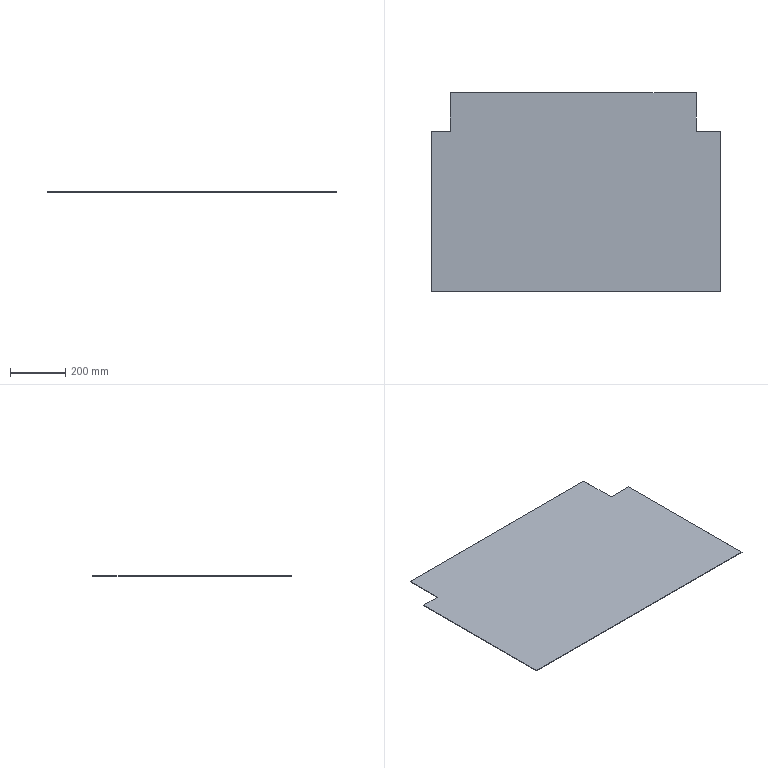Part | SolidWorks | 1 solid | 10 faces | box 1050 x 720 x 2 mm | volume 1467200 mm3 | plane 10
STEP:
#1=CARTESIAN_POINT('',(445.,655.,0.));
#2=VERTEX_POINT('',#1);
#3=CARTESIAN_POINT('',(445.,795.,0.));
#4=VERTEX_POINT('',#3);
#5=CARTESIAN_POINT('',(445.,795.,0.));
#6=DIRECTION('',(0.,1.,0.));
#7=VECTOR('',#6,1000.);
#8=LINE('',#5,#7);
#9=EDGE_CURVE('',#2,#4,#8,.T.);
#10=ORIENTED_EDGE('',*,*,#9,.T.);
#11=CARTESIAN_POINT('',(445.,795.,2.));
#12=VERTEX_POINT('',#11);
#13=CARTESIAN_POINT('',(445.,795.,2.));
#14=DIRECTION('',(0.,0.,-1.));
#15=VECTOR('',#14,1000.);
#16=LINE('',#13,#15);
#17=EDGE_CURVE('',#12,#4,#16,.T.);
#18=ORIENTED_EDGE('',*,*,#17,.F.);
#19=CARTESIAN_POINT('',(445.,655.,2.));
#20=VERTEX_POINT('',#19);
#21=CARTESIAN_POINT('',(445.,795.,2.));
#22=DIRECTION('',(0.,1.,0.));
#23=VECTOR('',#22,1000.);
#24=LINE('',#21,#23);
#25=EDGE_CURVE('',#20,#12,#24,.T.);
#26=ORIENTED_EDGE('',*,*,#25,.F.);
#27=CARTESIAN_POINT('',(445.,655.,2.));
#28=DIRECTION('',(0.,0.,-1.));
#29=VECTOR('',#28,1000.);
#30=LINE('',#27,#29);
#31=EDGE_CURVE('',#20,#2,#30,.T.);
#32=ORIENTED_EDGE('',*,*,#31,.T.);
#33=EDGE_LOOP('',(#10,#18,#26,#32));
#34=FACE_OUTER_BOUND('',#33,.T.);
#35=CARTESIAN_POINT('',(445.,795.,2.));
#36=DIRECTION('',(-1.,0.,0.));
#37=DIRECTION('',(0.,0.,1.));
#38=AXIS2_PLACEMENT_3D('',#35,#36,#37);
#39=PLANE('',#38);
#40=ADVANCED_FACE('',(#34),#39,.F.);
#41=CARTESIAN_POINT('',(-445.,795.,0.));
#42=VERTEX_POINT('',#41);
#43=CARTESIAN_POINT('',(-445.,795.,0.));
#44=DIRECTION('',(-1.,0.,0.));
#45=VECTOR('',#44,1000.);
#46=LINE('',#43,#45);
#47=EDGE_CURVE('',#4,#42,#46,.T.);
#48=ORIENTED_EDGE('',*,*,#47,.T.);
#49=CARTESIAN_POINT('',(-445.,795.,2.));
#50=VERTEX_POINT('',#49);
#51=CARTESIAN_POINT('',(-445.,795.,2.));
#52=DIRECTION('',(0.,0.,-1.));
#53=VECTOR('',#52,1000.);
#54=LINE('',#51,#53);
#55=EDGE_CURVE('',#50,#42,#54,.T.);
#56=ORIENTED_EDGE('',*,*,#55,.F.);
#57=CARTESIAN_POINT('',(-445.,795.,2.));
#58=DIRECTION('',(-1.,0.,0.));
#59=VECTOR('',#58,1000.);
#60=LINE('',#57,#59);
#61=EDGE_CURVE('',#12,#50,#60,.T.);
#62=ORIENTED_EDGE('',*,*,#61,.F.);
#63=ORIENTED_EDGE('',*,*,#17,.T.);
#64=EDGE_LOOP('',(#48,#56,#62,#63));
#65=FACE_OUTER_BOUND('',#64,.T.);
#66=CARTESIAN_POINT('',(-445.,795.,2.));
#67=DIRECTION('',(0.,-1.,0.));
#68=DIRECTION('',(0.,0.,-1.));
#69=AXIS2_PLACEMENT_3D('',#66,#67,#68);
#70=PLANE('',#69);
#71=ADVANCED_FACE('',(#65),#70,.F.);
#72=CARTESIAN_POINT('',(-445.,655.,0.));
#73=VERTEX_POINT('',#72);
#74=CARTESIAN_POINT('',(-445.,795.,0.));
#75=DIRECTION('',(0.,-1.,0.));
#76=VECTOR('',#75,1000.);
#77=LINE('',#74,#76);
#78=EDGE_CURVE('',#42,#73,#77,.T.);
#79=ORIENTED_EDGE('',*,*,#78,.T.);
#80=CARTESIAN_POINT('',(-445.,655.,2.));
#81=VERTEX_POINT('',#80);
#82=CARTESIAN_POINT('',(-445.,655.,2.));
#83=DIRECTION('',(0.,0.,-1.));
#84=VECTOR('',#83,1000.);
#85=LINE('',#82,#84);
#86=EDGE_CURVE('',#81,#73,#85,.T.);
#87=ORIENTED_EDGE('',*,*,#86,.F.);
#88=CARTESIAN_POINT('',(-445.,795.,2.));
#89=DIRECTION('',(0.,-1.,0.));
#90=VECTOR('',#89,1000.);
#91=LINE('',#88,#90);
#92=EDGE_CURVE('',#50,#81,#91,.T.);
#93=ORIENTED_EDGE('',*,*,#92,.F.);
#94=ORIENTED_EDGE('',*,*,#55,.T.);
#95=EDGE_LOOP('',(#79,#87,#93,#94));
#96=FACE_OUTER_BOUND('',#95,.T.);
#97=CARTESIAN_POINT('',(-445.,795.,2.));
#98=DIRECTION('',(1.,0.,0.));
#99=DIRECTION('',(0.,0.,-1.));
#100=AXIS2_PLACEMENT_3D('',#97,#98,#99);
#101=PLANE('',#100);
#102=ADVANCED_FACE('',(#96),#101,.F.);
#103=CARTESIAN_POINT('',(-515.,655.,0.));
#104=VERTEX_POINT('',#103);
#105=CARTESIAN_POINT('',(-445.,655.,0.));
#106=DIRECTION('',(-1.,0.,0.));
#107=VECTOR('',#106,1000.);
#108=LINE('',#105,#107);
#109=EDGE_CURVE('',#73,#104,#108,.T.);
#110=ORIENTED_EDGE('',*,*,#109,.T.);
#111=CARTESIAN_POINT('',(-515.,655.,2.));
#112=VERTEX_POINT('',#111);
#113=CARTESIAN_POINT('',(-515.,655.,2.));
#114=DIRECTION('',(0.,0.,-1.));
#115=VECTOR('',#114,1000.);
#116=LINE('',#113,#115);
#117=EDGE_CURVE('',#112,#104,#116,.T.);
#118=ORIENTED_EDGE('',*,*,#117,.F.);
#119=CARTESIAN_POINT('',(-445.,655.,2.));
#120=DIRECTION('',(-1.,0.,0.));
#121=VECTOR('',#120,1000.);
#122=LINE('',#119,#121);
#123=EDGE_CURVE('',#81,#112,#122,.T.);
#124=ORIENTED_EDGE('',*,*,#123,.F.);
#125=ORIENTED_EDGE('',*,*,#86,.T.);
#126=EDGE_LOOP('',(#110,#118,#124,#125));
#127=FACE_OUTER_BOUND('',#126,.T.);
#128=CARTESIAN_POINT('',(-445.,655.,2.));
#129=DIRECTION('',(0.,-1.,0.));
#130=DIRECTION('',(0.,0.,-1.));
#131=AXIS2_PLACEMENT_3D('',#128,#129,#130);
#132=PLANE('',#131);
#133=ADVANCED_FACE('',(#127),#132,.F.);
#134=CARTESIAN_POINT('',(-515.,75.,0.));
#135=VERTEX_POINT('',#134);
#136=CARTESIAN_POINT('',(-515.,655.,0.));
#137=DIRECTION('',(0.,-1.,0.));
#138=VECTOR('',#137,1000.);
#139=LINE('',#136,#138);
#140=EDGE_CURVE('',#104,#135,#139,.T.);
#141=ORIENTED_EDGE('',*,*,#140,.T.);
#142=CARTESIAN_POINT('',(-515.,75.,2.));
#143=VERTEX_POINT('',#142);
#144=CARTESIAN_POINT('',(-515.,75.,2.));
#145=DIRECTION('',(0.,0.,-1.));
#146=VECTOR('',#145,1000.);
#147=LINE('',#144,#146);
#148=EDGE_CURVE('',#143,#135,#147,.T.);
#149=ORIENTED_EDGE('',*,*,#148,.F.);
#150=CARTESIAN_POINT('',(-515.,655.,2.));
#151=DIRECTION('',(0.,-1.,0.));
#152=VECTOR('',#151,1000.);
#153=LINE('',#150,#152);
#154=EDGE_CURVE('',#112,#143,#153,.T.);
#155=ORIENTED_EDGE('',*,*,#154,.F.);
#156=ORIENTED_EDGE('',*,*,#117,.T.);
#157=EDGE_LOOP('',(#141,#149,#155,#156));
#158=FACE_OUTER_BOUND('',#157,.T.);
#159=CARTESIAN_POINT('',(-515.,655.,2.));
#160=DIRECTION('',(1.,0.,0.));
#161=DIRECTION('',(0.,1.,0.));
#162=AXIS2_PLACEMENT_3D('',#159,#160,#161);
#163=PLANE('',#162);
#164=ADVANCED_FACE('',(#158),#163,.F.);
#165=CARTESIAN_POINT('',(535.,75.,0.));
#166=VERTEX_POINT('',#165);
#167=CARTESIAN_POINT('',(-515.,75.,0.));
#168=DIRECTION('',(1.,0.,0.));
#169=VECTOR('',#168,1000.);
#170=LINE('',#167,#169);
#171=EDGE_CURVE('',#135,#166,#170,.T.);
#172=ORIENTED_EDGE('',*,*,#171,.T.);
#173=CARTESIAN_POINT('',(535.,75.,2.));
#174=VERTEX_POINT('',#173);
#175=CARTESIAN_POINT('',(535.,75.,2.));
#176=DIRECTION('',(0.,0.,-1.));
#177=VECTOR('',#176,1000.);
#178=LINE('',#175,#177);
#179=EDGE_CURVE('',#174,#166,#178,.T.);
#180=ORIENTED_EDGE('',*,*,#179,.F.);
#181=CARTESIAN_POINT('',(-515.,75.,2.));
#182=DIRECTION('',(1.,0.,0.));
#183=VECTOR('',#182,1000.);
#184=LINE('',#181,#183);
#185=EDGE_CURVE('',#143,#174,#184,.T.);
#186=ORIENTED_EDGE('',*,*,#185,.F.);
#187=ORIENTED_EDGE('',*,*,#148,.T.);
#188=EDGE_LOOP('',(#172,#180,#186,#187));
#189=FACE_OUTER_BOUND('',#188,.T.);
#190=CARTESIAN_POINT('',(-515.,75.,2.));
#191=DIRECTION('',(0.,1.,0.));
#192=DIRECTION('',(0.,0.,1.));
#193=AXIS2_PLACEMENT_3D('',#190,#191,#192);
#194=PLANE('',#193);
#195=ADVANCED_FACE('',(#189),#194,.F.);
#196=CARTESIAN_POINT('',(535.,655.,0.));
#197=VERTEX_POINT('',#196);
#198=CARTESIAN_POINT('',(535.,655.,0.));
#199=DIRECTION('',(0.,1.,0.));
#200=VECTOR('',#199,1000.);
#201=LINE('',#198,#200);
#202=EDGE_CURVE('',#166,#197,#201,.T.);
#203=ORIENTED_EDGE('',*,*,#202,.T.);
#204=CARTESIAN_POINT('',(535.,655.,2.));
#205=VERTEX_POINT('',#204);
#206=CARTESIAN_POINT('',(535.,655.,2.));
#207=DIRECTION('',(0.,0.,-1.));
#208=VECTOR('',#207,1000.);
#209=LINE('',#206,#208);
#210=EDGE_CURVE('',#205,#197,#209,.T.);
#211=ORIENTED_EDGE('',*,*,#210,.F.);
#212=CARTESIAN_POINT('',(535.,655.,2.));
#213=DIRECTION('',(0.,1.,0.));
#214=VECTOR('',#213,1000.);
#215=LINE('',#212,#214);
#216=EDGE_CURVE('',#174,#205,#215,.T.);
#217=ORIENTED_EDGE('',*,*,#216,.F.);
#218=ORIENTED_EDGE('',*,*,#179,.T.);
#219=EDGE_LOOP('',(#203,#211,#217,#218));
#220=FACE_OUTER_BOUND('',#219,.T.);
#221=CARTESIAN_POINT('',(535.,655.,2.));
#222=DIRECTION('',(-1.,0.,0.));
#223=DIRECTION('',(0.,-1.,0.));
#224=AXIS2_PLACEMENT_3D('',#221,#222,#223);
#225=PLANE('',#224);
#226=ADVANCED_FACE('',(#220),#225,.F.);
#227=CARTESIAN_POINT('',(445.,655.,0.));
#228=DIRECTION('',(-1.,0.,0.));
#229=VECTOR('',#228,1000.);
#230=LINE('',#227,#229);
#231=EDGE_CURVE('',#197,#2,#230,.T.);
#232=ORIENTED_EDGE('',*,*,#231,.T.);
#233=ORIENTED_EDGE('',*,*,#31,.F.);
#234=CARTESIAN_POINT('',(445.,655.,2.));
#235=DIRECTION('',(-1.,0.,0.));
#236=VECTOR('',#235,1000.);
#237=LINE('',#234,#236);
#238=EDGE_CURVE('',#205,#20,#237,.T.);
#239=ORIENTED_EDGE('',*,*,#238,.F.);
#240=ORIENTED_EDGE('',*,*,#210,.T.);
#241=EDGE_LOOP('',(#232,#233,#239,#240));
#242=FACE_OUTER_BOUND('',#241,.T.);
#243=CARTESIAN_POINT('',(445.,655.,2.));
#244=DIRECTION('',(0.,-1.,0.));
#245=DIRECTION('',(0.,0.,-1.));
#246=AXIS2_PLACEMENT_3D('',#243,#244,#245);
#247=PLANE('',#246);
#248=ADVANCED_FACE('',(#242),#247,.F.);
#249=ORIENTED_EDGE('',*,*,#25,.T.);
#250=ORIENTED_EDGE('',*,*,#61,.T.);
#251=ORIENTED_EDGE('',*,*,#92,.T.);
#252=ORIENTED_EDGE('',*,*,#123,.T.);
#253=ORIENTED_EDGE('',*,*,#154,.T.);
#254=ORIENTED_EDGE('',*,*,#185,.T.);
#255=ORIENTED_EDGE('',*,*,#216,.T.);
#256=ORIENTED_EDGE('',*,*,#238,.T.);
#257=EDGE_LOOP('',(#249,#250,#251,#252,#253,#254,#255,#256));
#258=FACE_OUTER_BOUND('',#257,.T.);
#259=CARTESIAN_POINT('',(0.,0.,2.));
#260=DIRECTION('',(0.,0.,1.));
#261=DIRECTION('',(1.,0.,0.));
#262=AXIS2_PLACEMENT_3D('',#259,#260,#261);
#263=PLANE('',#262);
#264=ADVANCED_FACE('',(#258),#263,.T.);
#265=ORIENTED_EDGE('',*,*,#9,.F.);
#266=ORIENTED_EDGE('',*,*,#231,.F.);
#267=ORIENTED_EDGE('',*,*,#202,.F.);
#268=ORIENTED_EDGE('',*,*,#171,.F.);
#269=ORIENTED_EDGE('',*,*,#140,.F.);
#270=ORIENTED_EDGE('',*,*,#109,.F.);
#271=ORIENTED_EDGE('',*,*,#78,.F.);
#272=ORIENTED_EDGE('',*,*,#47,.F.);
#273=EDGE_LOOP('',(#265,#266,#267,#268,#269,#270,#271,#272));
#274=FACE_OUTER_BOUND('',#273,.T.);
#275=CARTESIAN_POINT('',(0.,0.,0.));
#276=DIRECTION('',(0.,0.,1.));
#277=DIRECTION('',(1.,0.,0.));
#278=AXIS2_PLACEMENT_3D('',#275,#276,#277);
#279=PLANE('',#278);
#280=ADVANCED_FACE('',(#274),#279,.F.);
#281=CLOSED_SHELL('',(#40,#71,#102,#133,#164,#195,#226,#248,#264,#280));
#282=MANIFOLD_SOLID_BREP('',#281);
#283=CARTESIAN_POINT('',(0.,0.,0.));
#284=DIRECTION('',(0.,0.,1.));
#285=DIRECTION('',(1.,0.,0.));
#286=AXIS2_PLACEMENT_3D('',#283,#284,#285);
#287=(LENGTH_UNIT()NAMED_UNIT(*)SI_UNIT(.MILLI.,.METRE.));
#288=UNCERTAINTY_MEASURE_WITH_UNIT(LENGTH_MEASURE(0.00001),#287,'','');
#289=(NAMED_UNIT(*)PLANE_ANGLE_UNIT()SI_UNIT($,.RADIAN.));
#290=(NAMED_UNIT(*)SI_UNIT($,.STERADIAN.)SOLID_ANGLE_UNIT());
#291=(GEOMETRIC_REPRESENTATION_CONTEXT(3)GLOBAL_UNCERTAINTY_ASSIGNED_CONTEXT((#288))GLOBAL_UNIT_ASSIGNED_CONTEXT((#287,#289,#290))REPRESENTATION_CONTEXT('',''));
#292=ADVANCED_BREP_SHAPE_REPRESENTATION('',(#282,#286),#291);